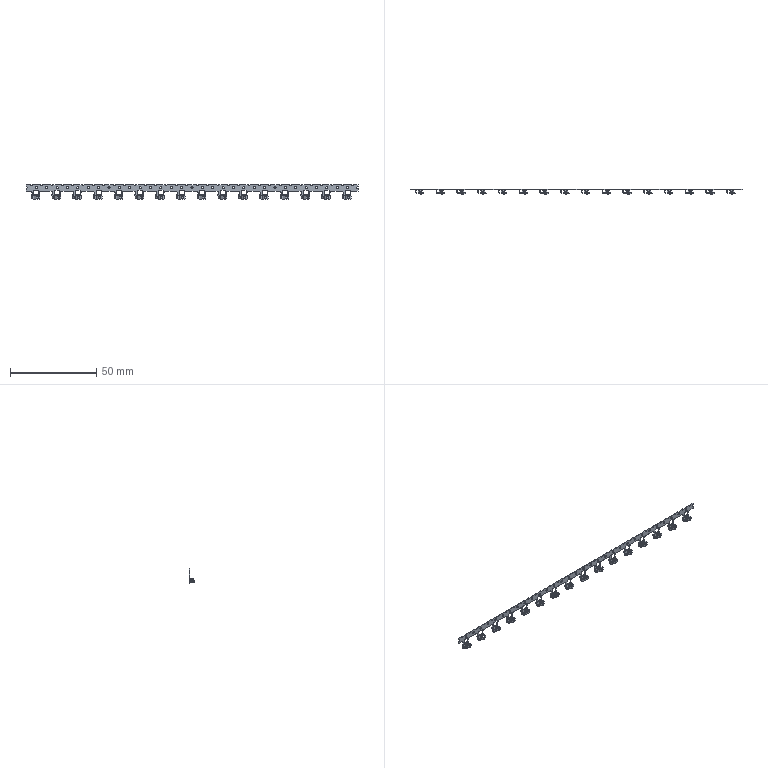Part | NX | 1 solid | 2761 faces | box 192 x 2.959 x 8.097 mm | volume 255.07 mm3 | plane 1656 | cylinder 881 | torus 192 | spline 32 | commonest cylinder face diameters 0.3 x256 0.2 x96 1.3 x81 0.5 x80 0.7 x80 0.35 x64